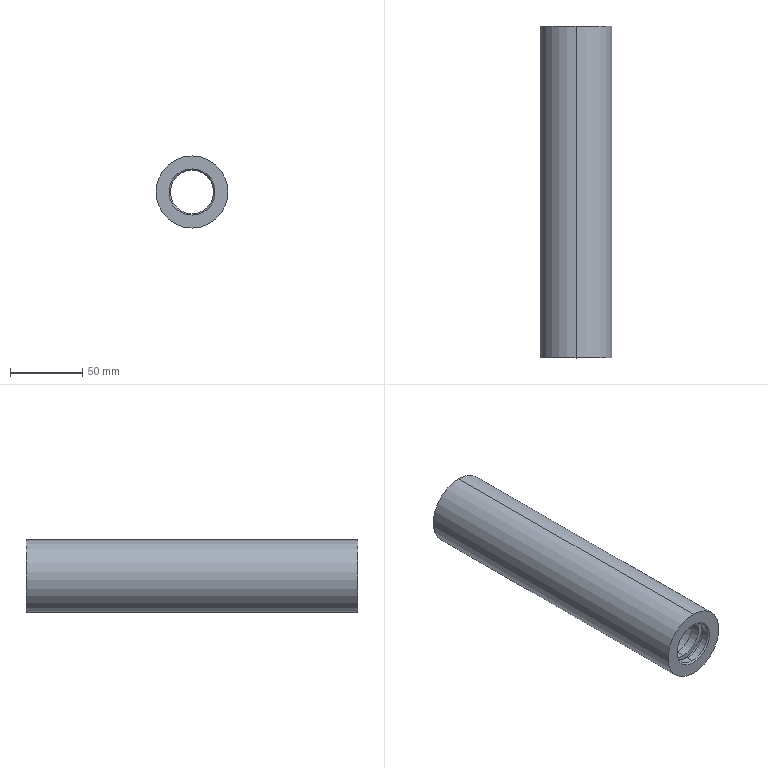Part | SolidWorks | features MirrorStock 1 | 1 solid | 28 faces | box 50 x 230 x 50 mm | volume 224751 mm3 | cylinder 16 | plane 8 | cone 4 | commonest cylinder face diameters 30 x8 36.54 x4 36 x2 50 x2
STEP:
#1=CARTESIAN_POINT('',(0.,229.,-15.));
#2=VERTEX_POINT('',#1);
#3=CARTESIAN_POINT('',(0.,229.,15.));
#4=VERTEX_POINT('',#3);
#5=CARTESIAN_POINT('',(0.,229.,0.));
#6=DIRECTION('',(0.,-1.,0.));
#7=DIRECTION('',(0.,0.,-1.));
#8=AXIS2_PLACEMENT_3D('',#5,#6,#7);
#9=CIRCLE('',#8,15.);
#10=EDGE_CURVE('',#2,#4,#9,.T.);
#11=ORIENTED_EDGE('',*,*,#10,.T.);
#12=CARTESIAN_POINT('',(0.,230.,16.));
#13=VERTEX_POINT('',#12);
#14=CARTESIAN_POINT('',(0.,230.,16.));
#15=DIRECTION('',(0.,0.7071,0.7071));
#16=VECTOR('',#15,1000.);
#17=LINE('',#14,#16);
#18=EDGE_CURVE('',#4,#13,#17,.T.);
#19=ORIENTED_EDGE('',*,*,#18,.T.);
#20=CARTESIAN_POINT('',(0.,230.,-16.));
#21=VERTEX_POINT('',#20);
#22=CARTESIAN_POINT('',(0.,230.,0.));
#23=DIRECTION('',(0.,1.,0.));
#24=DIRECTION('',(0.,0.,-1.));
#25=AXIS2_PLACEMENT_3D('',#22,#23,#24);
#26=CIRCLE('',#25,16.);
#27=EDGE_CURVE('',#13,#21,#26,.T.);
#28=ORIENTED_EDGE('',*,*,#27,.T.);
#29=CARTESIAN_POINT('',(0.,230.,-16.));
#30=DIRECTION('',(0.,0.7071,-0.7071));
#31=VECTOR('',#30,1000.);
#32=LINE('',#29,#31);
#33=EDGE_CURVE('',#2,#21,#32,.T.);
#34=ORIENTED_EDGE('',*,*,#33,.F.);
#35=EDGE_LOOP('',(#11,#19,#28,#34));
#36=FACE_OUTER_BOUND('',#35,.T.);
#37=CARTESIAN_POINT('',(0.,230.,0.));
#38=DIRECTION('',(0.,1.,0.));
#39=DIRECTION('',(0.,0.,-1.));
#40=AXIS2_PLACEMENT_3D('',#37,#38,#39);
#41=CONICAL_SURFACE('',#40,16.,0.7854);
#42=ADVANCED_FACE('',(#36),#41,.F.);
#43=CARTESIAN_POINT('',(0.,1.,15.));
#44=VERTEX_POINT('',#43);
#45=CARTESIAN_POINT('',(0.,1.,-15.));
#46=VERTEX_POINT('',#45);
#47=CARTESIAN_POINT('',(0.,1.,0.));
#48=DIRECTION('',(0.,1.,0.));
#49=DIRECTION('',(0.,0.,1.));
#50=AXIS2_PLACEMENT_3D('',#47,#48,#49);
#51=CIRCLE('',#50,15.);
#52=EDGE_CURVE('',#44,#46,#51,.T.);
#53=ORIENTED_EDGE('',*,*,#52,.T.);
#54=CARTESIAN_POINT('',(0.,0.,-16.));
#55=VERTEX_POINT('',#54);
#56=CARTESIAN_POINT('',(0.,1.,-15.));
#57=DIRECTION('',(0.,-0.7071,-0.7071));
#58=VECTOR('',#57,1000.);
#59=LINE('',#56,#58);
#60=EDGE_CURVE('',#46,#55,#59,.T.);
#61=ORIENTED_EDGE('',*,*,#60,.T.);
#62=CARTESIAN_POINT('',(0.,0.,16.));
#63=VERTEX_POINT('',#62);
#64=CARTESIAN_POINT('',(0.,0.,0.));
#65=DIRECTION('',(0.,-1.,0.));
#66=DIRECTION('',(0.,0.,1.));
#67=AXIS2_PLACEMENT_3D('',#64,#65,#66);
#68=CIRCLE('',#67,16.);
#69=EDGE_CURVE('',#55,#63,#68,.T.);
#70=ORIENTED_EDGE('',*,*,#69,.T.);
#71=CARTESIAN_POINT('',(0.,1.,15.));
#72=DIRECTION('',(0.,-0.7071,0.7071));
#73=VECTOR('',#72,1000.);
#74=LINE('',#71,#73);
#75=EDGE_CURVE('',#44,#63,#74,.T.);
#76=ORIENTED_EDGE('',*,*,#75,.F.);
#77=EDGE_LOOP('',(#53,#61,#70,#76));
#78=FACE_OUTER_BOUND('',#77,.T.);
#79=CARTESIAN_POINT('',(0.,1.,0.));
#80=DIRECTION('',(0.,-1.,0.));
#81=DIRECTION('',(0.,0.,1.));
#82=AXIS2_PLACEMENT_3D('',#79,#80,#81);
#83=CONICAL_SURFACE('',#82,15.,0.7854);
#84=ADVANCED_FACE('',(#78),#83,.F.);
#85=CARTESIAN_POINT('',(0.,9.8,18.27));
#86=VERTEX_POINT('',#85);
#87=CARTESIAN_POINT('',(0.,9.8,-18.27));
#88=VERTEX_POINT('',#87);
#89=CARTESIAN_POINT('',(0.,9.8,0.));
#90=DIRECTION('',(0.,1.,0.));
#91=DIRECTION('',(0.,0.,1.));
#92=AXIS2_PLACEMENT_3D('',#89,#90,#91);
#93=CIRCLE('',#92,18.27);
#94=EDGE_CURVE('',#86,#88,#93,.T.);
#95=ORIENTED_EDGE('',*,*,#94,.T.);
#96=CARTESIAN_POINT('',(0.,6.,-18.27));
#97=VERTEX_POINT('',#96);
#98=CARTESIAN_POINT('',(0.,0.,-18.27));
#99=DIRECTION('',(0.,-1.,0.));
#100=VECTOR('',#99,1000.);
#101=LINE('',#98,#100);
#102=EDGE_CURVE('',#88,#97,#101,.T.);
#103=ORIENTED_EDGE('',*,*,#102,.T.);
#104=CARTESIAN_POINT('',(0.,6.,18.27));
#105=VERTEX_POINT('',#104);
#106=CARTESIAN_POINT('',(0.,6.,0.));
#107=DIRECTION('',(0.,1.,0.));
#108=DIRECTION('',(0.,0.,1.));
#109=AXIS2_PLACEMENT_3D('',#106,#107,#108);
#110=CIRCLE('',#109,18.27);
#111=EDGE_CURVE('',#105,#97,#110,.T.);
#112=ORIENTED_EDGE('',*,*,#111,.F.);
#113=CARTESIAN_POINT('',(0.,0.,18.27));
#114=DIRECTION('',(0.,-1.,0.));
#115=VECTOR('',#114,1000.);
#116=LINE('',#113,#115);
#117=EDGE_CURVE('',#86,#105,#116,.T.);
#118=ORIENTED_EDGE('',*,*,#117,.F.);
#119=EDGE_LOOP('',(#95,#103,#112,#118));
#120=FACE_OUTER_BOUND('',#119,.T.);
#121=CARTESIAN_POINT('',(0.,0.,0.));
#122=DIRECTION('',(0.,-1.,0.));
#123=DIRECTION('',(0.,0.,1.));
#124=AXIS2_PLACEMENT_3D('',#121,#122,#123);
#125=CYLINDRICAL_SURFACE('',#124,18.27);
#126=ADVANCED_FACE('',(#120),#125,.F.);
#127=CARTESIAN_POINT('',(0.,16.,15.));
#128=VERTEX_POINT('',#127);
#129=CARTESIAN_POINT('',(0.,16.,-15.));
#130=VERTEX_POINT('',#129);
#131=CARTESIAN_POINT('',(0.,16.,0.));
#132=DIRECTION('',(0.,1.,0.));
#133=DIRECTION('',(0.,0.,1.));
#134=AXIS2_PLACEMENT_3D('',#131,#132,#133);
#135=CIRCLE('',#134,15.);
#136=EDGE_CURVE('',#128,#130,#135,.T.);
#137=ORIENTED_EDGE('',*,*,#136,.T.);
#138=CARTESIAN_POINT('',(0.,9.8,-15.));
#139=VERTEX_POINT('',#138);
#140=CARTESIAN_POINT('',(0.,0.,-15.));
#141=DIRECTION('',(0.,-1.,0.));
#142=VECTOR('',#141,1000.);
#143=LINE('',#140,#142);
#144=EDGE_CURVE('',#130,#139,#143,.T.);
#145=ORIENTED_EDGE('',*,*,#144,.T.);
#146=CARTESIAN_POINT('',(0.,9.8,15.));
#147=VERTEX_POINT('',#146);
#148=CARTESIAN_POINT('',(0.,9.8,0.));
#149=DIRECTION('',(0.,1.,0.));
#150=DIRECTION('',(0.,0.,1.));
#151=AXIS2_PLACEMENT_3D('',#148,#149,#150);
#152=CIRCLE('',#151,15.);
#153=EDGE_CURVE('',#147,#139,#152,.T.);
#154=ORIENTED_EDGE('',*,*,#153,.F.);
#155=CARTESIAN_POINT('',(0.,0.,15.));
#156=DIRECTION('',(0.,-1.,0.));
#157=VECTOR('',#156,1000.);
#158=LINE('',#155,#157);
#159=EDGE_CURVE('',#128,#147,#158,.T.);
#160=ORIENTED_EDGE('',*,*,#159,.F.);
#161=EDGE_LOOP('',(#137,#145,#154,#160));
#162=FACE_OUTER_BOUND('',#161,.T.);
#163=CARTESIAN_POINT('',(0.,0.,0.));
#164=DIRECTION('',(0.,-1.,0.));
#165=DIRECTION('',(0.,0.,1.));
#166=AXIS2_PLACEMENT_3D('',#163,#164,#165);
#167=CYLINDRICAL_SURFACE('',#166,15.);
#168=ADVANCED_FACE('',(#162),#167,.F.);
#169=CARTESIAN_POINT('',(0.,214.,18.));
#170=VERTEX_POINT('',#169);
#171=CARTESIAN_POINT('',(0.,214.,-18.));
#172=VERTEX_POINT('',#171);
#173=CARTESIAN_POINT('',(0.,214.,0.));
#174=DIRECTION('',(0.,1.,0.));
#175=DIRECTION('',(0.,0.,1.));
#176=AXIS2_PLACEMENT_3D('',#173,#174,#175);
#177=CIRCLE('',#176,18.);
#178=EDGE_CURVE('',#170,#172,#177,.T.);
#179=ORIENTED_EDGE('',*,*,#178,.T.);
#180=CARTESIAN_POINT('',(0.,16.,-18.));
#181=VERTEX_POINT('',#180);
#182=CARTESIAN_POINT('',(0.,0.,-18.));
#183=DIRECTION('',(0.,-1.,0.));
#184=VECTOR('',#183,1000.);
#185=LINE('',#182,#184);
#186=EDGE_CURVE('',#172,#181,#185,.T.);
#187=ORIENTED_EDGE('',*,*,#186,.T.);
#188=CARTESIAN_POINT('',(0.,16.,18.));
#189=VERTEX_POINT('',#188);
#190=CARTESIAN_POINT('',(0.,16.,0.));
#191=DIRECTION('',(0.,1.,0.));
#192=DIRECTION('',(0.,0.,1.));
#193=AXIS2_PLACEMENT_3D('',#190,#191,#192);
#194=CIRCLE('',#193,18.);
#195=EDGE_CURVE('',#189,#181,#194,.T.);
#196=ORIENTED_EDGE('',*,*,#195,.F.);
#197=CARTESIAN_POINT('',(0.,0.,18.));
#198=DIRECTION('',(0.,-1.,0.));
#199=VECTOR('',#198,1000.);
#200=LINE('',#197,#199);
#201=EDGE_CURVE('',#170,#189,#200,.T.);
#202=ORIENTED_EDGE('',*,*,#201,.F.);
#203=EDGE_LOOP('',(#179,#187,#196,#202));
#204=FACE_OUTER_BOUND('',#203,.T.);
#205=CARTESIAN_POINT('',(0.,0.,0.));
#206=DIRECTION('',(0.,-1.,0.));
#207=DIRECTION('',(0.,0.,1.));
#208=AXIS2_PLACEMENT_3D('',#205,#206,#207);
#209=CYLINDRICAL_SURFACE('',#208,18.);
#210=ADVANCED_FACE('',(#204),#209,.F.);
#211=CARTESIAN_POINT('',(0.,220.2,15.));
#212=VERTEX_POINT('',#211);
#213=CARTESIAN_POINT('',(0.,220.2,-15.));
#214=VERTEX_POINT('',#213);
#215=CARTESIAN_POINT('',(0.,220.2,0.));
#216=DIRECTION('',(0.,1.,0.));
#217=DIRECTION('',(0.,0.,1.));
#218=AXIS2_PLACEMENT_3D('',#215,#216,#217);
#219=CIRCLE('',#218,15.);
#220=EDGE_CURVE('',#212,#214,#219,.T.);
#221=ORIENTED_EDGE('',*,*,#220,.T.);
#222=CARTESIAN_POINT('',(0.,214.,-15.));
#223=VERTEX_POINT('',#222);
#224=CARTESIAN_POINT('',(0.,0.,-15.));
#225=DIRECTION('',(0.,-1.,0.));
#226=VECTOR('',#225,1000.);
#227=LINE('',#224,#226);
#228=EDGE_CURVE('',#214,#223,#227,.T.);
#229=ORIENTED_EDGE('',*,*,#228,.T.);
#230=CARTESIAN_POINT('',(0.,214.,15.));
#231=VERTEX_POINT('',#230);
#232=CARTESIAN_POINT('',(0.,214.,0.));
#233=DIRECTION('',(0.,1.,0.));
#234=DIRECTION('',(0.,0.,1.));
#235=AXIS2_PLACEMENT_3D('',#232,#233,#234);
#236=CIRCLE('',#235,15.);
#237=EDGE_CURVE('',#231,#223,#236,.T.);
#238=ORIENTED_EDGE('',*,*,#237,.F.);
#239=CARTESIAN_POINT('',(0.,0.,15.));
#240=DIRECTION('',(0.,-1.,0.));
#241=VECTOR('',#240,1000.);
#242=LINE('',#239,#241);
#243=EDGE_CURVE('',#212,#231,#242,.T.);
#244=ORIENTED_EDGE('',*,*,#243,.F.);
#245=EDGE_LOOP('',(#221,#229,#238,#244));
#246=FACE_OUTER_BOUND('',#245,.T.);
#247=CARTESIAN_POINT('',(0.,0.,0.));
#248=DIRECTION('',(0.,-1.,0.));
#249=DIRECTION('',(0.,0.,1.));
#250=AXIS2_PLACEMENT_3D('',#247,#248,#249);
#251=CYLINDRICAL_SURFACE('',#250,15.);
#252=ADVANCED_FACE('',(#246),#251,.F.);
#253=CARTESIAN_POINT('',(0.,224.,18.27));
#254=VERTEX_POINT('',#253);
#255=CARTESIAN_POINT('',(0.,224.,-18.27));
#256=VERTEX_POINT('',#255);
#257=CARTESIAN_POINT('',(0.,224.,0.));
#258=DIRECTION('',(0.,1.,0.));
#259=DIRECTION('',(0.,0.,1.));
#260=AXIS2_PLACEMENT_3D('',#257,#258,#259);
#261=CIRCLE('',#260,18.27);
#262=EDGE_CURVE('',#254,#256,#261,.T.);
#263=ORIENTED_EDGE('',*,*,#262,.T.);
#264=CARTESIAN_POINT('',(0.,220.2,-18.27));
#265=VERTEX_POINT('',#264);
#266=CARTESIAN_POINT('',(0.,0.,-18.27));
#267=DIRECTION('',(0.,-1.,0.));
#268=VECTOR('',#267,1000.);
#269=LINE('',#266,#268);
#270=EDGE_CURVE('',#256,#265,#269,.T.);
#271=ORIENTED_EDGE('',*,*,#270,.T.);
#272=CARTESIAN_POINT('',(0.,220.2,18.27));
#273=VERTEX_POINT('',#272);
#274=CARTESIAN_POINT('',(0.,220.2,0.));
#275=DIRECTION('',(0.,1.,0.));
#276=DIRECTION('',(0.,0.,1.));
#277=AXIS2_PLACEMENT_3D('',#274,#275,#276);
#278=CIRCLE('',#277,18.27);
#279=EDGE_CURVE('',#273,#265,#278,.T.);
#280=ORIENTED_EDGE('',*,*,#279,.F.);
#281=CARTESIAN_POINT('',(0.,0.,18.27));
#282=DIRECTION('',(0.,-1.,0.));
#283=VECTOR('',#282,1000.);
#284=LINE('',#281,#283);
#285=EDGE_CURVE('',#254,#273,#284,.T.);
#286=ORIENTED_EDGE('',*,*,#285,.F.);
#287=EDGE_LOOP('',(#263,#271,#280,#286));
#288=FACE_OUTER_BOUND('',#287,.T.);
#289=CARTESIAN_POINT('',(0.,0.,0.));
#290=DIRECTION('',(0.,-1.,0.));
#291=DIRECTION('',(0.,0.,1.));
#292=AXIS2_PLACEMENT_3D('',#289,#290,#291);
#293=CYLINDRICAL_SURFACE('',#292,18.27);
#294=ADVANCED_FACE('',(#288),#293,.F.);
#295=ORIENTED_EDGE('',*,*,#10,.F.);
#296=CARTESIAN_POINT('',(0.,224.,-15.));
#297=VERTEX_POINT('',#296);
#298=CARTESIAN_POINT('',(0.,0.,-15.));
#299=DIRECTION('',(0.,-1.,0.));
#300=VECTOR('',#299,1000.);
#301=LINE('',#298,#300);
#302=EDGE_CURVE('',#2,#297,#301,.T.);
#303=ORIENTED_EDGE('',*,*,#302,.T.);
#304=CARTESIAN_POINT('',(0.,224.,15.));
#305=VERTEX_POINT('',#304);
#306=CARTESIAN_POINT('',(0.,224.,0.));
#307=DIRECTION('',(0.,1.,0.));
#308=DIRECTION('',(0.,0.,1.));
#309=AXIS2_PLACEMENT_3D('',#306,#307,#308);
#310=CIRCLE('',#309,15.);
#311=EDGE_CURVE('',#305,#297,#310,.T.);
#312=ORIENTED_EDGE('',*,*,#311,.F.);
#313=CARTESIAN_POINT('',(0.,0.,15.));
#314=DIRECTION('',(0.,-1.,0.));
#315=VECTOR('',#314,1000.);
#316=LINE('',#313,#315);
#317=EDGE_CURVE('',#4,#305,#316,.T.);
#318=ORIENTED_EDGE('',*,*,#317,.F.);
#319=EDGE_LOOP('',(#295,#303,#312,#318));
#320=FACE_OUTER_BOUND('',#319,.T.);
#321=CARTESIAN_POINT('',(0.,0.,0.));
#322=DIRECTION('',(0.,-1.,0.));
#323=DIRECTION('',(0.,0.,1.));
#324=AXIS2_PLACEMENT_3D('',#321,#322,#323);
#325=CYLINDRICAL_SURFACE('',#324,15.);
#326=ADVANCED_FACE('',(#320),#325,.F.);
#327=CARTESIAN_POINT('',(0.,230.,-25.));
#328=VERTEX_POINT('',#327);
#329=CARTESIAN_POINT('',(0.,230.,25.));
#330=VERTEX_POINT('',#329);
#331=CARTESIAN_POINT('',(0.,230.,0.));
#332=DIRECTION('',(0.,1.,0.));
#333=DIRECTION('',(0.,0.,1.));
#334=AXIS2_PLACEMENT_3D('',#331,#332,#333);
#335=CIRCLE('',#334,25.);
#336=EDGE_CURVE('',#328,#330,#335,.T.);
#337=ORIENTED_EDGE('',*,*,#336,.F.);
#338=CARTESIAN_POINT('',(0.,0.,-25.));
#339=VERTEX_POINT('',#338);
#340=CARTESIAN_POINT('',(0.,0.,-25.));
#341=DIRECTION('',(0.,-1.,0.));
#342=VECTOR('',#341,1000.);
#343=LINE('',#340,#342);
#344=EDGE_CURVE('',#328,#339,#343,.T.);
#345=ORIENTED_EDGE('',*,*,#344,.T.);
#346=CARTESIAN_POINT('',(0.,0.,25.));
#347=VERTEX_POINT('',#346);
#348=CARTESIAN_POINT('',(0.,0.,0.));
#349=DIRECTION('',(0.,1.,0.));
#350=DIRECTION('',(0.,0.,1.));
#351=AXIS2_PLACEMENT_3D('',#348,#349,#350);
#352=CIRCLE('',#351,25.);
#353=EDGE_CURVE('',#339,#347,#352,.T.);
#354=ORIENTED_EDGE('',*,*,#353,.T.);
#355=CARTESIAN_POINT('',(0.,0.,25.));
#356=DIRECTION('',(0.,-1.,0.));
#357=VECTOR('',#356,1000.);
#358=LINE('',#355,#357);
#359=EDGE_CURVE('',#330,#347,#358,.T.);
#360=ORIENTED_EDGE('',*,*,#359,.F.);
#361=EDGE_LOOP('',(#337,#345,#354,#360));
#362=FACE_OUTER_BOUND('',#361,.T.);
#363=CARTESIAN_POINT('',(0.,0.,0.));
#364=DIRECTION('',(0.,-1.,0.));
#365=DIRECTION('',(0.,0.,1.));
#366=AXIS2_PLACEMENT_3D('',#363,#364,#365);
#367=CYLINDRICAL_SURFACE('',#366,25.);
#368=ADVANCED_FACE('',(#362),#367,.T.);
#369=CARTESIAN_POINT('',(0.,6.,15.));
#370=VERTEX_POINT('',#369);
#371=CARTESIAN_POINT('',(0.,6.,-15.));
#372=VERTEX_POINT('',#371);
#373=CARTESIAN_POINT('',(0.,6.,0.));
#374=DIRECTION('',(0.,1.,0.));
#375=DIRECTION('',(0.,0.,1.));
#376=AXIS2_PLACEMENT_3D('',#373,#374,#375);
#377=CIRCLE('',#376,15.);
#378=EDGE_CURVE('',#370,#372,#377,.T.);
#379=ORIENTED_EDGE('',*,*,#378,.T.);
#380=CARTESIAN_POINT('',(0.,0.,-15.));
#381=DIRECTION('',(0.,-1.,0.));
#382=VECTOR('',#381,1000.);
#383=LINE('',#380,#382);
#384=EDGE_CURVE('',#372,#46,#383,.T.);
#385=ORIENTED_EDGE('',*,*,#384,.T.);
#386=ORIENTED_EDGE('',*,*,#52,.F.);
#387=CARTESIAN_POINT('',(0.,0.,15.));
#388=DIRECTION('',(0.,-1.,0.));
#389=VECTOR('',#388,1000.);
#390=LINE('',#387,#389);
#391=EDGE_CURVE('',#370,#44,#390,.T.);
#392=ORIENTED_EDGE('',*,*,#391,.F.);
#393=EDGE_LOOP('',(#379,#385,#386,#392));
#394=FACE_OUTER_BOUND('',#393,.T.);
#395=CARTESIAN_POINT('',(0.,0.,0.));
#396=DIRECTION('',(0.,-1.,0.));
#397=DIRECTION('',(0.,0.,1.));
#398=AXIS2_PLACEMENT_3D('',#395,#396,#397);
#399=CYLINDRICAL_SURFACE('',#398,15.);
#400=ADVANCED_FACE('',(#394),#399,.F.);
#401=ORIENTED_EDGE('',*,*,#384,.F.);
#402=CARTESIAN_POINT('',(0.,6.,0.));
#403=DIRECTION('',(0.,1.,0.));
#404=DIRECTION('',(0.,0.,1.));
#405=AXIS2_PLACEMENT_3D('',#402,#403,#404);
#406=CIRCLE('',#405,15.);
#407=EDGE_CURVE('',#372,#370,#406,.T.);
#408=ORIENTED_EDGE('',*,*,#407,.T.);
#409=ORIENTED_EDGE('',*,*,#391,.T.);
#410=CARTESIAN_POINT('',(0.,1.,0.));
#411=DIRECTION('',(0.,1.,0.));
#412=DIRECTION('',(0.,0.,1.));
#413=AXIS2_PLACEMENT_3D('',#410,#411,#412);
#414=CIRCLE('',#413,15.);
#415=EDGE_CURVE('',#46,#44,#414,.T.);
#416=ORIENTED_EDGE('',*,*,#415,.F.);
#417=EDGE_LOOP('',(#401,#408,#409,#416));
#418=FACE_OUTER_BOUND('',#417,.T.);
#419=CARTESIAN_POINT('',(0.,0.,0.));
#420=DIRECTION('',(0.,-1.,0.));
#421=DIRECTION('',(0.,0.,1.));
#422=AXIS2_PLACEMENT_3D('',#419,#420,#421);
#423=CYLINDRICAL_SURFACE('',#422,15.);
#424=ADVANCED_FACE('',(#418),#423,.F.);
#425=CARTESIAN_POINT('',(0.,0.,0.));
#426=DIRECTION('',(0.,-1.,0.));
#427=DIRECTION('',(0.,0.,1.));
#428=AXIS2_PLACEMENT_3D('',#425,#426,#427);
#429=CIRCLE('',#428,16.);
#430=EDGE_CURVE('',#63,#55,#429,.T.);
#431=ORIENTED_EDGE('',*,*,#430,.F.);
#432=ORIENTED_EDGE('',*,*,#69,.F.);
#433=EDGE_LOOP('',(#431,#432));
#434=FACE_BOUND('',#433,.T.);
#435=CARTESIAN_POINT('',(0.,0.,0.));
#436=DIRECTION('',(0.,1.,0.));
#437=DIRECTION('',(0.,0.,1.));
#438=AXIS2_PLACEMENT_3D('',#435,#436,#437);
#439=CIRCLE('',#438,25.);
#440=EDGE_CURVE('',#347,#339,#439,.T.);
#441=ORIENTED_EDGE('',*,*,#440,.F.);
#442=ORIENTED_EDGE('',*,*,#353,.F.);
#443=EDGE_LOOP('',(#441,#442));
#444=FACE_OUTER_BOUND('',#443,.T.);
#445=CARTESIAN_POINT('',(0.,0.,0.));
#446=DIRECTION('',(0.,-1.,0.));
#447=DIRECTION('',(0.,0.,1.));
#448=AXIS2_PLACEMENT_3D('',#445,#446,#447);
#449=PLANE('',#448);
#450=ADVANCED_FACE('',(#434,#444),#449,.T.);
#451=ORIENTED_EDGE('',*,*,#344,.F.);
#452=CARTESIAN_POINT('',(0.,230.,0.));
#453=DIRECTION('',(0.,1.,0.));
#454=DIRECTION('',(0.,0.,1.));
#455=AXIS2_PLACEMENT_3D('',#452,#453,#454);
#456=CIRCLE('',#455,25.);
#457=EDGE_CURVE('',#330,#328,#456,.T.);
#458=ORIENTED_EDGE('',*,*,#457,.F.);
#459=ORIENTED_EDGE('',*,*,#359,.T.);
#460=ORIENTED_EDGE('',*,*,#440,.T.);
#461=EDGE_LOOP('',(#451,#458,#459,#460));
#462=FACE_OUTER_BOUND('',#461,.T.);
#463=CARTESIAN_POINT('',(0.,0.,0.));
#464=DIRECTION('',(0.,-1.,0.));
#465=DIRECTION('',(0.,0.,1.));
#466=AXIS2_PLACEMENT_3D('',#463,#464,#465);
#467=CYLINDRICAL_SURFACE('',#466,25.);
#468=ADVANCED_FACE('',(#462),#467,.T.);
#469=CARTESIAN_POINT('',(0.,230.,0.));
#470=DIRECTION('',(0.,1.,0.));
#471=DIRECTION('',(0.,0.,-1.));
#472=AXIS2_PLACEMENT_3D('',#469,#470,#471);
#473=CIRCLE('',#472,16.);
#474=EDGE_CURVE('',#21,#13,#473,.T.);
#475=ORIENTED_EDGE('',*,*,#474,.F.);
#476=ORIENTED_EDGE('',*,*,#27,.F.);
#477=EDGE_LOOP('',(#475,#476));
#478=FACE_BOUND('',#477,.T.);
#479=ORIENTED_EDGE('',*,*,#457,.T.);
#480=ORIENTED_EDGE('',*,*,#336,.T.);
#481=EDGE_LOOP('',(#479,#480));
#482=FACE_OUTER_BOUND('',#481,.T.);
#483=CARTESIAN_POINT('',(0.,230.,0.));
#484=DIRECTION('',(0.,1.,0.));
#485=DIRECTION('',(0.,0.,-1.));
#486=AXIS2_PLACEMENT_3D('',#483,#484,#485);
#487=PLANE('',#486);
#488=ADVANCED_FACE('',(#478,#482),#487,.T.);
#489=ORIENTED_EDGE('',*,*,#302,.F.);
#490=CARTESIAN_POINT('',(0.,229.,0.));
#491=DIRECTION('',(0.,-1.,0.));
#492=DIRECTION('',(0.,0.,-1.));
#493=AXIS2_PLACEMENT_3D('',#490,#491,#492);
#494=CIRCLE('',#493,15.);
#495=EDGE_CURVE('',#4,#2,#494,.T.);
#496=ORIENTED_EDGE('',*,*,#495,.F.);
#497=ORIENTED_EDGE('',*,*,#317,.T.);
#498=CARTESIAN_POINT('',(0.,224.,0.));
#499=DIRECTION('',(0.,1.,0.));
#500=DIRECTION('',(0.,0.,1.));
#501=AXIS2_PLACEMENT_3D('',#498,#499,#500);
#502=CIRCLE('',#501,15.);
#503=EDGE_CURVE('',#297,#305,#502,.T.);
#504=ORIENTED_EDGE('',*,*,#503,.F.);
#505=EDGE_LOOP('',(#489,#496,#497,#504));
#506=FACE_OUTER_BOUND('',#505,.T.);
#507=CARTESIAN_POINT('',(0.,0.,0.));
#508=DIRECTION('',(0.,-1.,0.));
#509=DIRECTION('',(0.,0.,1.));
#510=AXIS2_PLACEMENT_3D('',#507,#508,#509);
#511=CYLINDRICAL_SURFACE('',#510,15.);
#512=ADVANCED_FACE('',(#506),#511,.F.);
#513=ORIENTED_EDGE('',*,*,#262,.F.);
#514=CARTESIAN_POINT('',(0.,224.,0.));
#515=DIRECTION('',(0.,1.,0.));
#516=DIRECTION('',(0.,0.,1.));
#517=AXIS2_PLACEMENT_3D('',#514,#515,#516);
#518=CIRCLE('',#517,18.27);
#519=EDGE_CURVE('',#256,#254,#518,.T.);
#520=ORIENTED_EDGE('',*,*,#519,.F.);
#521=EDGE_LOOP('',(#513,#520));
#522=FACE_OUTER_BOUND('',#521,.T.);
#523=ORIENTED_EDGE('',*,*,#311,.T.);
#524=ORIENTED_EDGE('',*,*,#503,.T.);
#525=EDGE_LOOP('',(#523,#524));
#526=FACE_BOUND('',#525,.T.);
#527=CARTESIAN_POINT('',(0.,224.,0.));
#528=DIRECTION('',(0.,-1.,0.));
#529=DIRECTION('',(0.,0.,1.));
#530=AXIS2_PLACEMENT_3D('',#527,#528,#529);
#531=PLANE('',#530);
#532=ADVANCED_FACE('',(#522,#526),#531,.T.);
#533=ORIENTED_EDGE('',*,*,#270,.F.);
#534=ORIENTED_EDGE('',*,*,#519,.T.);
#535=ORIENTED_EDGE('',*,*,#285,.T.);
#536=CARTESIAN_POINT('',(0.,220.2,0.));
#537=DIRECTION('',(0.,1.,0.));
#538=DIRECTION('',(0.,0.,1.));
#539=AXIS2_PLACEMENT_3D('',#536,#537,#538);
#540=CIRCLE('',#539,18.27);
#541=EDGE_CURVE('',#265,#273,#540,.T.);
#542=ORIENTED_EDGE('',*,*,#541,.F.);
#543=EDGE_LOOP('',(#533,#534,#535,#542));
#544=FACE_OUTER_BOUND('',#543,.T.);
#545=CARTESIAN_POINT('',(0.,0.,0.));
#546=DIRECTION('',(0.,-1.,0.));
#547=DIRECTION('',(0.,0.,1.));
#548=AXIS2_PLACEMENT_3D('',#545,#546,#547);
#549=CYLINDRICAL_SURFACE('',#548,18.27);
#550=ADVANCED_FACE('',(#544),#549,.F.);
#551=ORIENTED_EDGE('',*,*,#220,.F.);
#552=CARTESIAN_POINT('',(0.,220.2,0.));
#553=DIRECTION('',(0.,1.,0.));
#554=DIRECTION('',(0.,0.,1.));
#555=AXIS2_PLACEMENT_3D('',#552,#553,#554);
#556=CIRCLE('',#555,15.);
#557=EDGE_CURVE('',#214,#212,#556,.T.);
#558=ORIENTED_EDGE('',*,*,#557,.F.);
#559=EDGE_LOOP('',(#551,#558));
#560=FACE_BOUND('',#559,.T.);
#561=ORIENTED_EDGE('',*,*,#279,.T.);
#562=ORIENTED_EDGE('',*,*,#541,.T.);
#563=EDGE_LOOP('',(#561,#562));
#564=FACE_OUTER_BOUND('',#563,.T.);
#565=CARTESIAN_POINT('',(0.,220.2,0.));
#566=DIRECTION('',(0.,1.,0.));
#567=DIRECTION('',(0.,0.,-1.));
#568=AXIS2_PLACEMENT_3D('',#565,#566,#567);
#569=PLANE('',#568);
#570=ADVANCED_FACE('',(#560,#564),#569,.T.);
#571=ORIENTED_EDGE('',*,*,#228,.F.);
#572=ORIENTED_EDGE('',*,*,#557,.T.);
#573=ORIENTED_EDGE('',*,*,#243,.T.);
#574=CARTESIAN_POINT('',(0.,214.,0.));
#575=DIRECTION('',(0.,1.,0.));
#576=DIRECTION('',(0.,0.,1.));
#577=AXIS2_PLACEMENT_3D('',#574,#575,#576);
#578=CIRCLE('',#577,15.);
#579=EDGE_CURVE('',#223,#231,#578,.T.);
#580=ORIENTED_EDGE('',*,*,#579,.F.);
#581=EDGE_LOOP('',(#571,#572,#573,#580));
#582=FACE_OUTER_BOUND('',#581,.T.);
#583=CARTESIAN_POINT('',(0.,0.,0.));
#584=DIRECTION('',(0.,-1.,0.));
#585=DIRECTION('',(0.,0.,1.));
#586=AXIS2_PLACEMENT_3D('',#583,#584,#585);
#587=CYLINDRICAL_SURFACE('',#586,15.);
#588=ADVANCED_FACE('',(#582),#587,.F.);
#589=ORIENTED_EDGE('',*,*,#178,.F.);
#590=CARTESIAN_POINT('',(0.,214.,0.));
#591=DIRECTION('',(0.,1.,0.));
#592=DIRECTION('',(0.,0.,1.));
#593=AXIS2_PLACEMENT_3D('',#590,#591,#592);
#594=CIRCLE('',#593,18.);
#595=EDGE_CURVE('',#172,#170,#594,.T.);
#596=ORIENTED_EDGE('',*,*,#595,.F.);
#597=EDGE_LOOP('',(#589,#596));
#598=FACE_OUTER_BOUND('',#597,.T.);
#599=ORIENTED_EDGE('',*,*,#237,.T.);
#600=ORIENTED_EDGE('',*,*,#579,.T.);
#601=EDGE_LOOP('',(#599,#600));
#602=FACE_BOUND('',#601,.T.);
#603=CARTESIAN_POINT('',(0.,214.,0.));
#604=DIRECTION('',(0.,-1.,0.));
#605=DIRECTION('',(0.,0.,1.));
#606=AXIS2_PLACEMENT_3D('',#603,#604,#605);
#607=PLANE('',#606);
#608=ADVANCED_FACE('',(#598,#602),#607,.T.);
#609=ORIENTED_EDGE('',*,*,#186,.F.);
#610=ORIENTED_EDGE('',*,*,#595,.T.);
#611=ORIENTED_EDGE('',*,*,#201,.T.);
#612=CARTESIAN_POINT('',(0.,16.,0.));
#613=DIRECTION('',(0.,1.,0.));
#614=DIRECTION('',(0.,0.,1.));
#615=AXIS2_PLACEMENT_3D('',#612,#613,#614);
#616=CIRCLE('',#615,18.);
#617=EDGE_CURVE('',#181,#189,#616,.T.);
#618=ORIENTED_EDGE('',*,*,#617,.F.);
#619=EDGE_LOOP('',(#609,#610,#611,#618));
#620=FACE_OUTER_BOUND('',#619,.T.);
#621=CARTESIAN_POINT('',(0.,0.,0.));
#622=DIRECTION('',(0.,-1.,0.));
#623=DIRECTION('',(0.,0.,1.));
#624=AXIS2_PLACEMENT_3D('',#621,#622,#623);
#625=CYLINDRICAL_SURFACE('',#624,18.);
#626=ADVANCED_FACE('',(#620),#625,.F.);
#627=ORIENTED_EDGE('',*,*,#195,.T.);
#628=ORIENTED_EDGE('',*,*,#617,.T.);
#629=EDGE_LOOP('',(#627,#628));
#630=FACE_OUTER_BOUND('',#629,.T.);
#631=ORIENTED_EDGE('',*,*,#136,.F.);
#632=CARTESIAN_POINT('',(0.,16.,0.));
#633=DIRECTION('',(0.,1.,0.));
#634=DIRECTION('',(0.,0.,1.));
#635=AXIS2_PLACEMENT_3D('',#632,#633,#634);
#636=CIRCLE('',#635,15.);
#637=EDGE_CURVE('',#130,#128,#636,.T.);
#638=ORIENTED_EDGE('',*,*,#637,.F.);
#639=EDGE_LOOP('',(#631,#638));
#640=FACE_BOUND('',#639,.T.);
#641=CARTESIAN_POINT('',(0.,16.,0.));
#642=DIRECTION('',(0.,-1.,0.));
#643=DIRECTION('',(0.,0.,1.));
#644=AXIS2_PLACEMENT_3D('',#641,#642,#643);
#645=PLANE('',#644);
#646=ADVANCED_FACE('',(#630,#640),#645,.F.);
#647=ORIENTED_EDGE('',*,*,#144,.F.);
#648=ORIENTED_EDGE('',*,*,#637,.T.);
#649=ORIENTED_EDGE('',*,*,#159,.T.);
#650=CARTESIAN_POINT('',(0.,9.8,0.));
#651=DIRECTION('',(0.,1.,0.));
#652=DIRECTION('',(0.,0.,1.));
#653=AXIS2_PLACEMENT_3D('',#650,#651,#652);
#654=CIRCLE('',#653,15.);
#655=EDGE_CURVE('',#139,#147,#654,.T.);
#656=ORIENTED_EDGE('',*,*,#655,.F.);
#657=EDGE_LOOP('',(#647,#648,#649,#656));
#658=FACE_OUTER_BOUND('',#657,.T.);
#659=CARTESIAN_POINT('',(0.,0.,0.));
#660=DIRECTION('',(0.,-1.,0.));
#661=DIRECTION('',(0.,0.,1.));
#662=AXIS2_PLACEMENT_3D('',#659,#660,#661);
#663=CYLINDRICAL_SURFACE('',#662,15.);
#664=ADVANCED_FACE('',(#658),#663,.F.);
#665=ORIENTED_EDGE('',*,*,#153,.T.);
#666=ORIENTED_EDGE('',*,*,#655,.T.);
#667=EDGE_LOOP('',(#665,#666));
#668=FACE_BOUND('',#667,.T.);
#669=ORIENTED_EDGE('',*,*,#94,.F.);
#670=CARTESIAN_POINT('',(0.,9.8,0.));
#671=DIRECTION('',(0.,1.,0.));
#672=DIRECTION('',(0.,0.,1.));
#673=AXIS2_PLACEMENT_3D('',#670,#671,#672);
#674=CIRCLE('',#673,18.27);
#675=EDGE_CURVE('',#88,#86,#674,.T.);
#676=ORIENTED_EDGE('',*,*,#675,.F.);
#677=EDGE_LOOP('',(#669,#676));
#678=FACE_OUTER_BOUND('',#677,.T.);
#679=CARTESIAN_POINT('',(0.,9.8,0.));
#680=DIRECTION('',(0.,1.,0.));
#681=DIRECTION('',(0.,0.,-1.));
#682=AXIS2_PLACEMENT_3D('',#679,#680,#681);
#683=PLANE('',#682);
#684=ADVANCED_FACE('',(#668,#678),#683,.F.);
#685=ORIENTED_EDGE('',*,*,#102,.F.);
#686=ORIENTED_EDGE('',*,*,#675,.T.);
#687=ORIENTED_EDGE('',*,*,#117,.T.);
#688=CARTESIAN_POINT('',(0.,6.,0.));
#689=DIRECTION('',(0.,1.,0.));
#690=DIRECTION('',(0.,0.,1.));
#691=AXIS2_PLACEMENT_3D('',#688,#689,#690);
#692=CIRCLE('',#691,18.27);
#693=EDGE_CURVE('',#97,#105,#692,.T.);
#694=ORIENTED_EDGE('',*,*,#693,.F.);
#695=EDGE_LOOP('',(#685,#686,#687,#694));
#696=FACE_OUTER_BOUND('',#695,.T.);
#697=CARTESIAN_POINT('',(0.,0.,0.));
#698=DIRECTION('',(0.,-1.,0.));
#699=DIRECTION('',(0.,0.,1.));
#700=AXIS2_PLACEMENT_3D('',#697,#698,#699);
#701=CYLINDRICAL_SURFACE('',#700,18.27);
#702=ADVANCED_FACE('',(#696),#701,.F.);
#703=ORIENTED_EDGE('',*,*,#111,.T.);
#704=ORIENTED_EDGE('',*,*,#693,.T.);
#705=EDGE_LOOP('',(#703,#704));
#706=FACE_OUTER_BOUND('',#705,.T.);
#707=ORIENTED_EDGE('',*,*,#378,.F.);
#708=ORIENTED_EDGE('',*,*,#407,.F.);
#709=EDGE_LOOP('',(#707,#708));
#710=FACE_BOUND('',#709,.T.);
#711=CARTESIAN_POINT('',(0.,6.,0.));
#712=DIRECTION('',(0.,-1.,0.));
#713=DIRECTION('',(0.,0.,1.));
#714=AXIS2_PLACEMENT_3D('',#711,#712,#713);
#715=PLANE('',#714);
#716=ADVANCED_FACE('',(#706,#710),#715,.F.);
#717=ORIENTED_EDGE('',*,*,#60,.F.);
#718=ORIENTED_EDGE('',*,*,#415,.T.);
#719=ORIENTED_EDGE('',*,*,#75,.T.);
#720=ORIENTED_EDGE('',*,*,#430,.T.);
#721=EDGE_LOOP('',(#717,#718,#719,#720));
#722=FACE_OUTER_BOUND('',#721,.T.);
#723=CARTESIAN_POINT('',(0.,1.,0.));
#724=DIRECTION('',(0.,-1.,0.));
#725=DIRECTION('',(0.,0.,1.));
#726=AXIS2_PLACEMENT_3D('',#723,#724,#725);
#727=CONICAL_SURFACE('',#726,15.,0.7854);
#728=ADVANCED_FACE('',(#722),#727,.F.);
#729=ORIENTED_EDGE('',*,*,#18,.F.);
#730=ORIENTED_EDGE('',*,*,#495,.T.);
#731=ORIENTED_EDGE('',*,*,#33,.T.);
#732=ORIENTED_EDGE('',*,*,#474,.T.);
#733=EDGE_LOOP('',(#729,#730,#731,#732));
#734=FACE_OUTER_BOUND('',#733,.T.);
#735=CARTESIAN_POINT('',(0.,230.,0.));
#736=DIRECTION('',(0.,1.,0.));
#737=DIRECTION('',(0.,0.,-1.));
#738=AXIS2_PLACEMENT_3D('',#735,#736,#737);
#739=CONICAL_SURFACE('',#738,16.,0.7854);
#740=ADVANCED_FACE('',(#734),#739,.F.);
#741=CLOSED_SHELL('',(#42,#84,#126,#168,#210,#252,#294,#326,#368,#400,#424,#450,#468,#488,#512,#532,#550,#570,#588,#608,#626,#646,#664,#684,#702,#716,#728,#740));
#742=MANIFOLD_SOLID_BREP('',#741);
#743=CARTESIAN_POINT('',(0.,0.,0.));
#744=DIRECTION('',(0.,0.,1.));
#745=DIRECTION('',(1.,0.,0.));
#746=AXIS2_PLACEMENT_3D('',#743,#744,#745);
#747=(LENGTH_UNIT()NAMED_UNIT(*)SI_UNIT(.MILLI.,.METRE.));
#748=UNCERTAINTY_MEASURE_WITH_UNIT(LENGTH_MEASURE(0.00001),#747,'','');
#749=(NAMED_UNIT(*)PLANE_ANGLE_UNIT()SI_UNIT($,.RADIAN.));
#750=(NAMED_UNIT(*)SI_UNIT($,.STERADIAN.)SOLID_ANGLE_UNIT());
#751=(GEOMETRIC_REPRESENTATION_CONTEXT(3)GLOBAL_UNCERTAINTY_ASSIGNED_CONTEXT((#748))GLOBAL_UNIT_ASSIGNED_CONTEXT((#747,#749,#750))REPRESENTATION_CONTEXT('',''));
#752=ADVANCED_BREP_SHAPE_REPRESENTATION('',(#742,#746),#751);